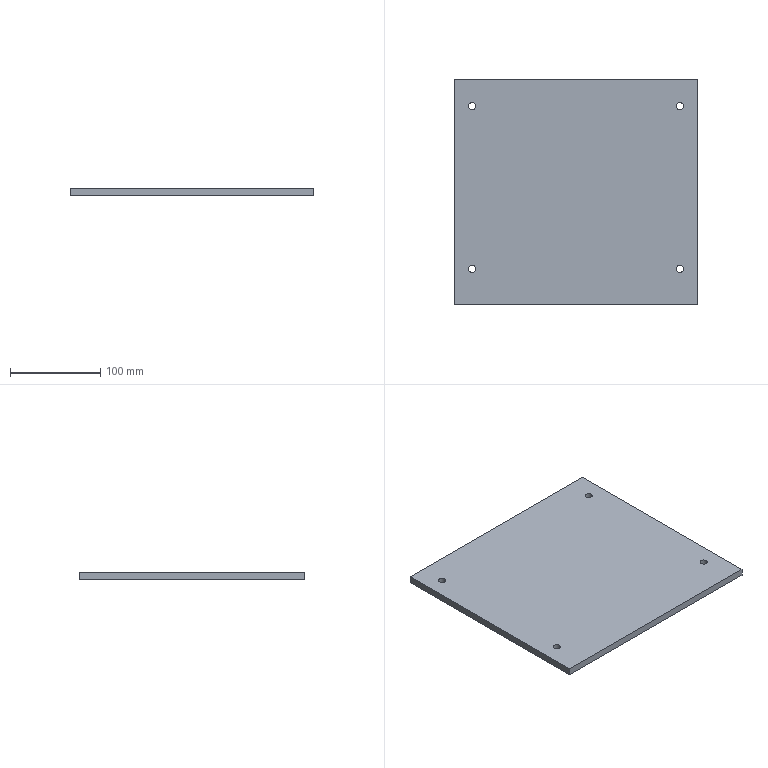Part | SolidWorks | features Cut 1, Extrusion 1 | 1 solid | 14 faces | box 270 x 250 x 8 mm | volume 538392 mm3 | cylinder 8 | plane 6 | commonest cylinder face diameters 8 x8
STEP:
#1=CARTESIAN_POINT('',(24.,-210.,0.));
#2=VERTEX_POINT('',#1);
#3=CARTESIAN_POINT('',(16.,-210.,0.));
#4=VERTEX_POINT('',#3);
#5=CARTESIAN_POINT('',(20.,-210.,0.));
#6=DIRECTION('',(0.,0.,-1.));
#7=DIRECTION('',(-1.,0.,0.));
#8=AXIS2_PLACEMENT_3D('',#5,#6,#7);
#9=CIRCLE('',#8,4.);
#10=EDGE_CURVE('',#2,#4,#9,.T.);
#11=ORIENTED_EDGE('',*,*,#10,.T.);
#12=CARTESIAN_POINT('',(16.,-210.,8.));
#13=VERTEX_POINT('',#12);
#14=CARTESIAN_POINT('',(16.,-210.,-2.));
#15=DIRECTION('',(0.,0.,1.));
#16=VECTOR('',#15,1000.);
#17=LINE('',#14,#16);
#18=EDGE_CURVE('',#4,#13,#17,.T.);
#19=ORIENTED_EDGE('',*,*,#18,.T.);
#20=CARTESIAN_POINT('',(24.,-210.,8.));
#21=VERTEX_POINT('',#20);
#22=CARTESIAN_POINT('',(20.,-210.,8.));
#23=DIRECTION('',(0.,0.,1.));
#24=DIRECTION('',(1.,0.,0.));
#25=AXIS2_PLACEMENT_3D('',#22,#23,#24);
#26=CIRCLE('',#25,4.);
#27=EDGE_CURVE('',#13,#21,#26,.T.);
#28=ORIENTED_EDGE('',*,*,#27,.T.);
#29=CARTESIAN_POINT('',(24.,-210.,-2.));
#30=DIRECTION('',(0.,0.,1.));
#31=VECTOR('',#30,1000.);
#32=LINE('',#29,#31);
#33=EDGE_CURVE('',#2,#21,#32,.T.);
#34=ORIENTED_EDGE('',*,*,#33,.F.);
#35=EDGE_LOOP('',(#11,#19,#28,#34));
#36=FACE_OUTER_BOUND('',#35,.T.);
#37=CARTESIAN_POINT('',(20.,-210.,-2.));
#38=DIRECTION('',(0.,0.,1.));
#39=DIRECTION('',(1.,0.,0.));
#40=AXIS2_PLACEMENT_3D('',#37,#38,#39);
#41=CYLINDRICAL_SURFACE('',#40,4.);
#42=ADVANCED_FACE('',(#36),#41,.F.);
#43=CARTESIAN_POINT('',(24.,-30.,0.));
#44=VERTEX_POINT('',#43);
#45=CARTESIAN_POINT('',(16.,-30.,0.));
#46=VERTEX_POINT('',#45);
#47=CARTESIAN_POINT('',(20.,-30.,0.));
#48=DIRECTION('',(0.,0.,-1.));
#49=DIRECTION('',(-1.,0.,0.));
#50=AXIS2_PLACEMENT_3D('',#47,#48,#49);
#51=CIRCLE('',#50,4.);
#52=EDGE_CURVE('',#44,#46,#51,.T.);
#53=ORIENTED_EDGE('',*,*,#52,.T.);
#54=CARTESIAN_POINT('',(16.,-30.,8.));
#55=VERTEX_POINT('',#54);
#56=CARTESIAN_POINT('',(16.,-30.,-2.));
#57=DIRECTION('',(0.,0.,1.));
#58=VECTOR('',#57,1000.);
#59=LINE('',#56,#58);
#60=EDGE_CURVE('',#46,#55,#59,.T.);
#61=ORIENTED_EDGE('',*,*,#60,.T.);
#62=CARTESIAN_POINT('',(24.,-30.,8.));
#63=VERTEX_POINT('',#62);
#64=CARTESIAN_POINT('',(20.,-30.,8.));
#65=DIRECTION('',(0.,0.,1.));
#66=DIRECTION('',(1.,0.,0.));
#67=AXIS2_PLACEMENT_3D('',#64,#65,#66);
#68=CIRCLE('',#67,4.);
#69=EDGE_CURVE('',#55,#63,#68,.T.);
#70=ORIENTED_EDGE('',*,*,#69,.T.);
#71=CARTESIAN_POINT('',(24.,-30.,-2.));
#72=DIRECTION('',(0.,0.,1.));
#73=VECTOR('',#72,1000.);
#74=LINE('',#71,#73);
#75=EDGE_CURVE('',#44,#63,#74,.T.);
#76=ORIENTED_EDGE('',*,*,#75,.F.);
#77=EDGE_LOOP('',(#53,#61,#70,#76));
#78=FACE_OUTER_BOUND('',#77,.T.);
#79=CARTESIAN_POINT('',(20.,-30.,-2.));
#80=DIRECTION('',(0.,0.,1.));
#81=DIRECTION('',(1.,0.,0.));
#82=AXIS2_PLACEMENT_3D('',#79,#80,#81);
#83=CYLINDRICAL_SURFACE('',#82,4.);
#84=ADVANCED_FACE('',(#78),#83,.F.);
#85=CARTESIAN_POINT('',(254.,-30.,0.));
#86=VERTEX_POINT('',#85);
#87=CARTESIAN_POINT('',(246.,-30.,0.));
#88=VERTEX_POINT('',#87);
#89=CARTESIAN_POINT('',(250.,-30.,0.));
#90=DIRECTION('',(0.,0.,-1.));
#91=DIRECTION('',(-1.,0.,0.));
#92=AXIS2_PLACEMENT_3D('',#89,#90,#91);
#93=CIRCLE('',#92,4.);
#94=EDGE_CURVE('',#86,#88,#93,.T.);
#95=ORIENTED_EDGE('',*,*,#94,.T.);
#96=CARTESIAN_POINT('',(246.,-30.,8.));
#97=VERTEX_POINT('',#96);
#98=CARTESIAN_POINT('',(246.,-30.,-2.));
#99=DIRECTION('',(0.,0.,1.));
#100=VECTOR('',#99,1000.);
#101=LINE('',#98,#100);
#102=EDGE_CURVE('',#88,#97,#101,.T.);
#103=ORIENTED_EDGE('',*,*,#102,.T.);
#104=CARTESIAN_POINT('',(254.,-30.,8.));
#105=VERTEX_POINT('',#104);
#106=CARTESIAN_POINT('',(250.,-30.,8.));
#107=DIRECTION('',(0.,0.,1.));
#108=DIRECTION('',(1.,0.,0.));
#109=AXIS2_PLACEMENT_3D('',#106,#107,#108);
#110=CIRCLE('',#109,4.);
#111=EDGE_CURVE('',#97,#105,#110,.T.);
#112=ORIENTED_EDGE('',*,*,#111,.T.);
#113=CARTESIAN_POINT('',(254.,-30.,-2.));
#114=DIRECTION('',(0.,0.,1.));
#115=VECTOR('',#114,1000.);
#116=LINE('',#113,#115);
#117=EDGE_CURVE('',#86,#105,#116,.T.);
#118=ORIENTED_EDGE('',*,*,#117,.F.);
#119=EDGE_LOOP('',(#95,#103,#112,#118));
#120=FACE_OUTER_BOUND('',#119,.T.);
#121=CARTESIAN_POINT('',(250.,-30.,-2.));
#122=DIRECTION('',(0.,0.,1.));
#123=DIRECTION('',(1.,0.,0.));
#124=AXIS2_PLACEMENT_3D('',#121,#122,#123);
#125=CYLINDRICAL_SURFACE('',#124,4.);
#126=ADVANCED_FACE('',(#120),#125,.F.);
#127=CARTESIAN_POINT('',(254.,-210.,0.));
#128=VERTEX_POINT('',#127);
#129=CARTESIAN_POINT('',(246.,-210.,0.));
#130=VERTEX_POINT('',#129);
#131=CARTESIAN_POINT('',(250.,-210.,0.));
#132=DIRECTION('',(0.,0.,-1.));
#133=DIRECTION('',(-1.,0.,0.));
#134=AXIS2_PLACEMENT_3D('',#131,#132,#133);
#135=CIRCLE('',#134,4.);
#136=EDGE_CURVE('',#128,#130,#135,.T.);
#137=ORIENTED_EDGE('',*,*,#136,.T.);
#138=CARTESIAN_POINT('',(246.,-210.,8.));
#139=VERTEX_POINT('',#138);
#140=CARTESIAN_POINT('',(246.,-210.,-2.));
#141=DIRECTION('',(0.,0.,1.));
#142=VECTOR('',#141,1000.);
#143=LINE('',#140,#142);
#144=EDGE_CURVE('',#130,#139,#143,.T.);
#145=ORIENTED_EDGE('',*,*,#144,.T.);
#146=CARTESIAN_POINT('',(254.,-210.,8.));
#147=VERTEX_POINT('',#146);
#148=CARTESIAN_POINT('',(250.,-210.,8.));
#149=DIRECTION('',(0.,0.,1.));
#150=DIRECTION('',(1.,0.,0.));
#151=AXIS2_PLACEMENT_3D('',#148,#149,#150);
#152=CIRCLE('',#151,4.);
#153=EDGE_CURVE('',#139,#147,#152,.T.);
#154=ORIENTED_EDGE('',*,*,#153,.T.);
#155=CARTESIAN_POINT('',(254.,-210.,-2.));
#156=DIRECTION('',(0.,0.,1.));
#157=VECTOR('',#156,1000.);
#158=LINE('',#155,#157);
#159=EDGE_CURVE('',#128,#147,#158,.T.);
#160=ORIENTED_EDGE('',*,*,#159,.F.);
#161=EDGE_LOOP('',(#137,#145,#154,#160));
#162=FACE_OUTER_BOUND('',#161,.T.);
#163=CARTESIAN_POINT('',(250.,-210.,-2.));
#164=DIRECTION('',(0.,0.,1.));
#165=DIRECTION('',(1.,0.,0.));
#166=AXIS2_PLACEMENT_3D('',#163,#164,#165);
#167=CYLINDRICAL_SURFACE('',#166,4.);
#168=ADVANCED_FACE('',(#162),#167,.F.);
#169=CARTESIAN_POINT('',(0.,0.,0.));
#170=VERTEX_POINT('',#169);
#171=CARTESIAN_POINT('',(0.,-250.,0.));
#172=VERTEX_POINT('',#171);
#173=CARTESIAN_POINT('',(0.,-250.,0.));
#174=DIRECTION('',(0.,-1.,0.));
#175=VECTOR('',#174,1000.);
#176=LINE('',#173,#175);
#177=EDGE_CURVE('',#170,#172,#176,.T.);
#178=ORIENTED_EDGE('',*,*,#177,.T.);
#179=CARTESIAN_POINT('',(0.,-250.,8.));
#180=VERTEX_POINT('',#179);
#181=CARTESIAN_POINT('',(0.,-250.,8.));
#182=DIRECTION('',(0.,0.,-1.));
#183=VECTOR('',#182,1000.);
#184=LINE('',#181,#183);
#185=EDGE_CURVE('',#180,#172,#184,.T.);
#186=ORIENTED_EDGE('',*,*,#185,.F.);
#187=CARTESIAN_POINT('',(0.,0.,8.));
#188=VERTEX_POINT('',#187);
#189=CARTESIAN_POINT('',(0.,-250.,8.));
#190=DIRECTION('',(0.,-1.,0.));
#191=VECTOR('',#190,1000.);
#192=LINE('',#189,#191);
#193=EDGE_CURVE('',#188,#180,#192,.T.);
#194=ORIENTED_EDGE('',*,*,#193,.F.);
#195=CARTESIAN_POINT('',(0.,0.,8.));
#196=DIRECTION('',(0.,0.,-1.));
#197=VECTOR('',#196,1000.);
#198=LINE('',#195,#197);
#199=EDGE_CURVE('',#188,#170,#198,.T.);
#200=ORIENTED_EDGE('',*,*,#199,.T.);
#201=EDGE_LOOP('',(#178,#186,#194,#200));
#202=FACE_OUTER_BOUND('',#201,.T.);
#203=CARTESIAN_POINT('',(0.,-250.,8.));
#204=DIRECTION('',(1.,0.,0.));
#205=DIRECTION('',(0.,0.,-1.));
#206=AXIS2_PLACEMENT_3D('',#203,#204,#205);
#207=PLANE('',#206);
#208=ADVANCED_FACE('',(#202),#207,.F.);
#209=CARTESIAN_POINT('',(270.,-250.,0.));
#210=VERTEX_POINT('',#209);
#211=CARTESIAN_POINT('',(270.,-250.,0.));
#212=DIRECTION('',(1.,0.,0.));
#213=VECTOR('',#212,1000.);
#214=LINE('',#211,#213);
#215=EDGE_CURVE('',#172,#210,#214,.T.);
#216=ORIENTED_EDGE('',*,*,#215,.T.);
#217=CARTESIAN_POINT('',(270.,-250.,8.));
#218=VERTEX_POINT('',#217);
#219=CARTESIAN_POINT('',(270.,-250.,8.));
#220=DIRECTION('',(0.,0.,-1.));
#221=VECTOR('',#220,1000.);
#222=LINE('',#219,#221);
#223=EDGE_CURVE('',#218,#210,#222,.T.);
#224=ORIENTED_EDGE('',*,*,#223,.F.);
#225=CARTESIAN_POINT('',(270.,-250.,8.));
#226=DIRECTION('',(1.,0.,0.));
#227=VECTOR('',#226,1000.);
#228=LINE('',#225,#227);
#229=EDGE_CURVE('',#180,#218,#228,.T.);
#230=ORIENTED_EDGE('',*,*,#229,.F.);
#231=ORIENTED_EDGE('',*,*,#185,.T.);
#232=EDGE_LOOP('',(#216,#224,#230,#231));
#233=FACE_OUTER_BOUND('',#232,.T.);
#234=CARTESIAN_POINT('',(270.,-250.,8.));
#235=DIRECTION('',(0.,1.,0.));
#236=DIRECTION('',(0.,0.,1.));
#237=AXIS2_PLACEMENT_3D('',#234,#235,#236);
#238=PLANE('',#237);
#239=ADVANCED_FACE('',(#233),#238,.F.);
#240=CARTESIAN_POINT('',(270.,0.,0.));
#241=VERTEX_POINT('',#240);
#242=CARTESIAN_POINT('',(270.,0.,0.));
#243=DIRECTION('',(0.,1.,0.));
#244=VECTOR('',#243,1000.);
#245=LINE('',#242,#244);
#246=EDGE_CURVE('',#210,#241,#245,.T.);
#247=ORIENTED_EDGE('',*,*,#246,.T.);
#248=CARTESIAN_POINT('',(270.,0.,8.));
#249=VERTEX_POINT('',#248);
#250=CARTESIAN_POINT('',(270.,0.,8.));
#251=DIRECTION('',(0.,0.,-1.));
#252=VECTOR('',#251,1000.);
#253=LINE('',#250,#252);
#254=EDGE_CURVE('',#249,#241,#253,.T.);
#255=ORIENTED_EDGE('',*,*,#254,.F.);
#256=CARTESIAN_POINT('',(270.,0.,8.));
#257=DIRECTION('',(0.,1.,0.));
#258=VECTOR('',#257,1000.);
#259=LINE('',#256,#258);
#260=EDGE_CURVE('',#218,#249,#259,.T.);
#261=ORIENTED_EDGE('',*,*,#260,.F.);
#262=ORIENTED_EDGE('',*,*,#223,.T.);
#263=EDGE_LOOP('',(#247,#255,#261,#262));
#264=FACE_OUTER_BOUND('',#263,.T.);
#265=CARTESIAN_POINT('',(270.,0.,8.));
#266=DIRECTION('',(-1.,0.,0.));
#267=DIRECTION('',(0.,-1.,0.));
#268=AXIS2_PLACEMENT_3D('',#265,#266,#267);
#269=PLANE('',#268);
#270=ADVANCED_FACE('',(#264),#269,.F.);
#271=CARTESIAN_POINT('',(0.,0.,0.));
#272=DIRECTION('',(-1.,0.,0.));
#273=VECTOR('',#272,1000.);
#274=LINE('',#271,#273);
#275=EDGE_CURVE('',#241,#170,#274,.T.);
#276=ORIENTED_EDGE('',*,*,#275,.T.);
#277=ORIENTED_EDGE('',*,*,#199,.F.);
#278=CARTESIAN_POINT('',(0.,0.,8.));
#279=DIRECTION('',(-1.,0.,0.));
#280=VECTOR('',#279,1000.);
#281=LINE('',#278,#280);
#282=EDGE_CURVE('',#249,#188,#281,.T.);
#283=ORIENTED_EDGE('',*,*,#282,.F.);
#284=ORIENTED_EDGE('',*,*,#254,.T.);
#285=EDGE_LOOP('',(#276,#277,#283,#284));
#286=FACE_OUTER_BOUND('',#285,.T.);
#287=CARTESIAN_POINT('',(0.,0.,8.));
#288=DIRECTION('',(0.,-1.,0.));
#289=DIRECTION('',(0.,0.,-1.));
#290=AXIS2_PLACEMENT_3D('',#287,#288,#289);
#291=PLANE('',#290);
#292=ADVANCED_FACE('',(#286),#291,.F.);
#293=CARTESIAN_POINT('',(20.,-210.,8.));
#294=DIRECTION('',(0.,0.,1.));
#295=DIRECTION('',(1.,0.,0.));
#296=AXIS2_PLACEMENT_3D('',#293,#294,#295);
#297=CIRCLE('',#296,4.);
#298=EDGE_CURVE('',#21,#13,#297,.T.);
#299=ORIENTED_EDGE('',*,*,#298,.F.);
#300=ORIENTED_EDGE('',*,*,#27,.F.);
#301=EDGE_LOOP('',(#299,#300));
#302=FACE_BOUND('',#301,.T.);
#303=CARTESIAN_POINT('',(20.,-30.,8.));
#304=DIRECTION('',(0.,0.,1.));
#305=DIRECTION('',(1.,0.,0.));
#306=AXIS2_PLACEMENT_3D('',#303,#304,#305);
#307=CIRCLE('',#306,4.);
#308=EDGE_CURVE('',#63,#55,#307,.T.);
#309=ORIENTED_EDGE('',*,*,#308,.F.);
#310=ORIENTED_EDGE('',*,*,#69,.F.);
#311=EDGE_LOOP('',(#309,#310));
#312=FACE_BOUND('',#311,.T.);
#313=CARTESIAN_POINT('',(250.,-30.,8.));
#314=DIRECTION('',(0.,0.,1.));
#315=DIRECTION('',(1.,0.,0.));
#316=AXIS2_PLACEMENT_3D('',#313,#314,#315);
#317=CIRCLE('',#316,4.);
#318=EDGE_CURVE('',#105,#97,#317,.T.);
#319=ORIENTED_EDGE('',*,*,#318,.F.);
#320=ORIENTED_EDGE('',*,*,#111,.F.);
#321=EDGE_LOOP('',(#319,#320));
#322=FACE_BOUND('',#321,.T.);
#323=CARTESIAN_POINT('',(250.,-210.,8.));
#324=DIRECTION('',(0.,0.,1.));
#325=DIRECTION('',(1.,0.,0.));
#326=AXIS2_PLACEMENT_3D('',#323,#324,#325);
#327=CIRCLE('',#326,4.);
#328=EDGE_CURVE('',#147,#139,#327,.T.);
#329=ORIENTED_EDGE('',*,*,#328,.F.);
#330=ORIENTED_EDGE('',*,*,#153,.F.);
#331=EDGE_LOOP('',(#329,#330));
#332=FACE_BOUND('',#331,.T.);
#333=ORIENTED_EDGE('',*,*,#193,.T.);
#334=ORIENTED_EDGE('',*,*,#229,.T.);
#335=ORIENTED_EDGE('',*,*,#260,.T.);
#336=ORIENTED_EDGE('',*,*,#282,.T.);
#337=EDGE_LOOP('',(#333,#334,#335,#336));
#338=FACE_OUTER_BOUND('',#337,.T.);
#339=CARTESIAN_POINT('',(0.,0.,8.));
#340=DIRECTION('',(0.,0.,-1.));
#341=DIRECTION('',(-1.,0.,0.));
#342=AXIS2_PLACEMENT_3D('',#339,#340,#341);
#343=PLANE('',#342);
#344=ADVANCED_FACE('',(#302,#312,#322,#332,#338),#343,.F.);
#345=ORIENTED_EDGE('',*,*,#10,.F.);
#346=CARTESIAN_POINT('',(20.,-210.,0.));
#347=DIRECTION('',(0.,0.,-1.));
#348=DIRECTION('',(-1.,0.,0.));
#349=AXIS2_PLACEMENT_3D('',#346,#347,#348);
#350=CIRCLE('',#349,4.);
#351=EDGE_CURVE('',#4,#2,#350,.T.);
#352=ORIENTED_EDGE('',*,*,#351,.F.);
#353=EDGE_LOOP('',(#345,#352));
#354=FACE_BOUND('',#353,.T.);
#355=ORIENTED_EDGE('',*,*,#52,.F.);
#356=CARTESIAN_POINT('',(20.,-30.,0.));
#357=DIRECTION('',(0.,0.,-1.));
#358=DIRECTION('',(-1.,0.,0.));
#359=AXIS2_PLACEMENT_3D('',#356,#357,#358);
#360=CIRCLE('',#359,4.);
#361=EDGE_CURVE('',#46,#44,#360,.T.);
#362=ORIENTED_EDGE('',*,*,#361,.F.);
#363=EDGE_LOOP('',(#355,#362));
#364=FACE_BOUND('',#363,.T.);
#365=ORIENTED_EDGE('',*,*,#94,.F.);
#366=CARTESIAN_POINT('',(250.,-30.,0.));
#367=DIRECTION('',(0.,0.,-1.));
#368=DIRECTION('',(-1.,0.,0.));
#369=AXIS2_PLACEMENT_3D('',#366,#367,#368);
#370=CIRCLE('',#369,4.);
#371=EDGE_CURVE('',#88,#86,#370,.T.);
#372=ORIENTED_EDGE('',*,*,#371,.F.);
#373=EDGE_LOOP('',(#365,#372));
#374=FACE_BOUND('',#373,.T.);
#375=ORIENTED_EDGE('',*,*,#136,.F.);
#376=CARTESIAN_POINT('',(250.,-210.,0.));
#377=DIRECTION('',(0.,0.,-1.));
#378=DIRECTION('',(-1.,0.,0.));
#379=AXIS2_PLACEMENT_3D('',#376,#377,#378);
#380=CIRCLE('',#379,4.);
#381=EDGE_CURVE('',#130,#128,#380,.T.);
#382=ORIENTED_EDGE('',*,*,#381,.F.);
#383=EDGE_LOOP('',(#375,#382));
#384=FACE_BOUND('',#383,.T.);
#385=ORIENTED_EDGE('',*,*,#177,.F.);
#386=ORIENTED_EDGE('',*,*,#275,.F.);
#387=ORIENTED_EDGE('',*,*,#246,.F.);
#388=ORIENTED_EDGE('',*,*,#215,.F.);
#389=EDGE_LOOP('',(#385,#386,#387,#388));
#390=FACE_OUTER_BOUND('',#389,.T.);
#391=CARTESIAN_POINT('',(0.,0.,0.));
#392=DIRECTION('',(0.,0.,-1.));
#393=DIRECTION('',(-1.,0.,0.));
#394=AXIS2_PLACEMENT_3D('',#391,#392,#393);
#395=PLANE('',#394);
#396=ADVANCED_FACE('',(#354,#364,#374,#384,#390),#395,.T.);
#397=ORIENTED_EDGE('',*,*,#144,.F.);
#398=ORIENTED_EDGE('',*,*,#381,.T.);
#399=ORIENTED_EDGE('',*,*,#159,.T.);
#400=ORIENTED_EDGE('',*,*,#328,.T.);
#401=EDGE_LOOP('',(#397,#398,#399,#400));
#402=FACE_OUTER_BOUND('',#401,.T.);
#403=CARTESIAN_POINT('',(250.,-210.,-2.));
#404=DIRECTION('',(0.,0.,1.));
#405=DIRECTION('',(1.,0.,0.));
#406=AXIS2_PLACEMENT_3D('',#403,#404,#405);
#407=CYLINDRICAL_SURFACE('',#406,4.);
#408=ADVANCED_FACE('',(#402),#407,.F.);
#409=ORIENTED_EDGE('',*,*,#102,.F.);
#410=ORIENTED_EDGE('',*,*,#371,.T.);
#411=ORIENTED_EDGE('',*,*,#117,.T.);
#412=ORIENTED_EDGE('',*,*,#318,.T.);
#413=EDGE_LOOP('',(#409,#410,#411,#412));
#414=FACE_OUTER_BOUND('',#413,.T.);
#415=CARTESIAN_POINT('',(250.,-30.,-2.));
#416=DIRECTION('',(0.,0.,1.));
#417=DIRECTION('',(1.,0.,0.));
#418=AXIS2_PLACEMENT_3D('',#415,#416,#417);
#419=CYLINDRICAL_SURFACE('',#418,4.);
#420=ADVANCED_FACE('',(#414),#419,.F.);
#421=ORIENTED_EDGE('',*,*,#60,.F.);
#422=ORIENTED_EDGE('',*,*,#361,.T.);
#423=ORIENTED_EDGE('',*,*,#75,.T.);
#424=ORIENTED_EDGE('',*,*,#308,.T.);
#425=EDGE_LOOP('',(#421,#422,#423,#424));
#426=FACE_OUTER_BOUND('',#425,.T.);
#427=CARTESIAN_POINT('',(20.,-30.,-2.));
#428=DIRECTION('',(0.,0.,1.));
#429=DIRECTION('',(1.,0.,0.));
#430=AXIS2_PLACEMENT_3D('',#427,#428,#429);
#431=CYLINDRICAL_SURFACE('',#430,4.);
#432=ADVANCED_FACE('',(#426),#431,.F.);
#433=ORIENTED_EDGE('',*,*,#18,.F.);
#434=ORIENTED_EDGE('',*,*,#351,.T.);
#435=ORIENTED_EDGE('',*,*,#33,.T.);
#436=ORIENTED_EDGE('',*,*,#298,.T.);
#437=EDGE_LOOP('',(#433,#434,#435,#436));
#438=FACE_OUTER_BOUND('',#437,.T.);
#439=CARTESIAN_POINT('',(20.,-210.,-2.));
#440=DIRECTION('',(0.,0.,1.));
#441=DIRECTION('',(1.,0.,0.));
#442=AXIS2_PLACEMENT_3D('',#439,#440,#441);
#443=CYLINDRICAL_SURFACE('',#442,4.);
#444=ADVANCED_FACE('',(#438),#443,.F.);
#445=CLOSED_SHELL('',(#42,#84,#126,#168,#208,#239,#270,#292,#344,#396,#408,#420,#432,#444));
#446=MANIFOLD_SOLID_BREP('',#445);
#447=CARTESIAN_POINT('',(0.,0.,0.));
#448=DIRECTION('',(0.,0.,1.));
#449=DIRECTION('',(1.,0.,0.));
#450=AXIS2_PLACEMENT_3D('',#447,#448,#449);
#451=(LENGTH_UNIT()NAMED_UNIT(*)SI_UNIT(.MILLI.,.METRE.));
#452=UNCERTAINTY_MEASURE_WITH_UNIT(LENGTH_MEASURE(0.00001),#451,'','');
#453=(NAMED_UNIT(*)PLANE_ANGLE_UNIT()SI_UNIT($,.RADIAN.));
#454=(NAMED_UNIT(*)SI_UNIT($,.STERADIAN.)SOLID_ANGLE_UNIT());
#455=(GEOMETRIC_REPRESENTATION_CONTEXT(3)GLOBAL_UNCERTAINTY_ASSIGNED_CONTEXT((#452))GLOBAL_UNIT_ASSIGNED_CONTEXT((#451,#453,#454))REPRESENTATION_CONTEXT('',''));
#456=ADVANCED_BREP_SHAPE_REPRESENTATION('',(#446,#450),#455);